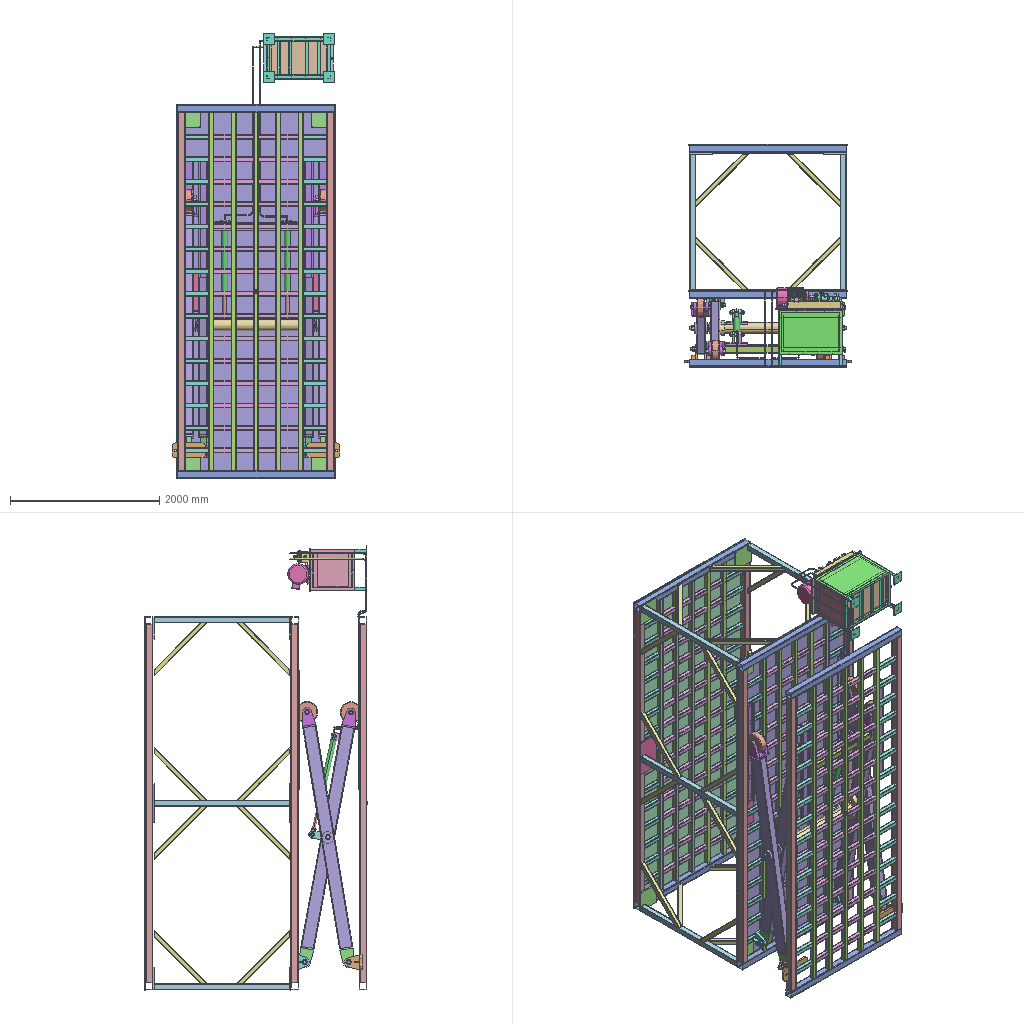Assembly | SolidWorks | 68 different items | 528 placed | box 2250 x 2986 x 5966 mm
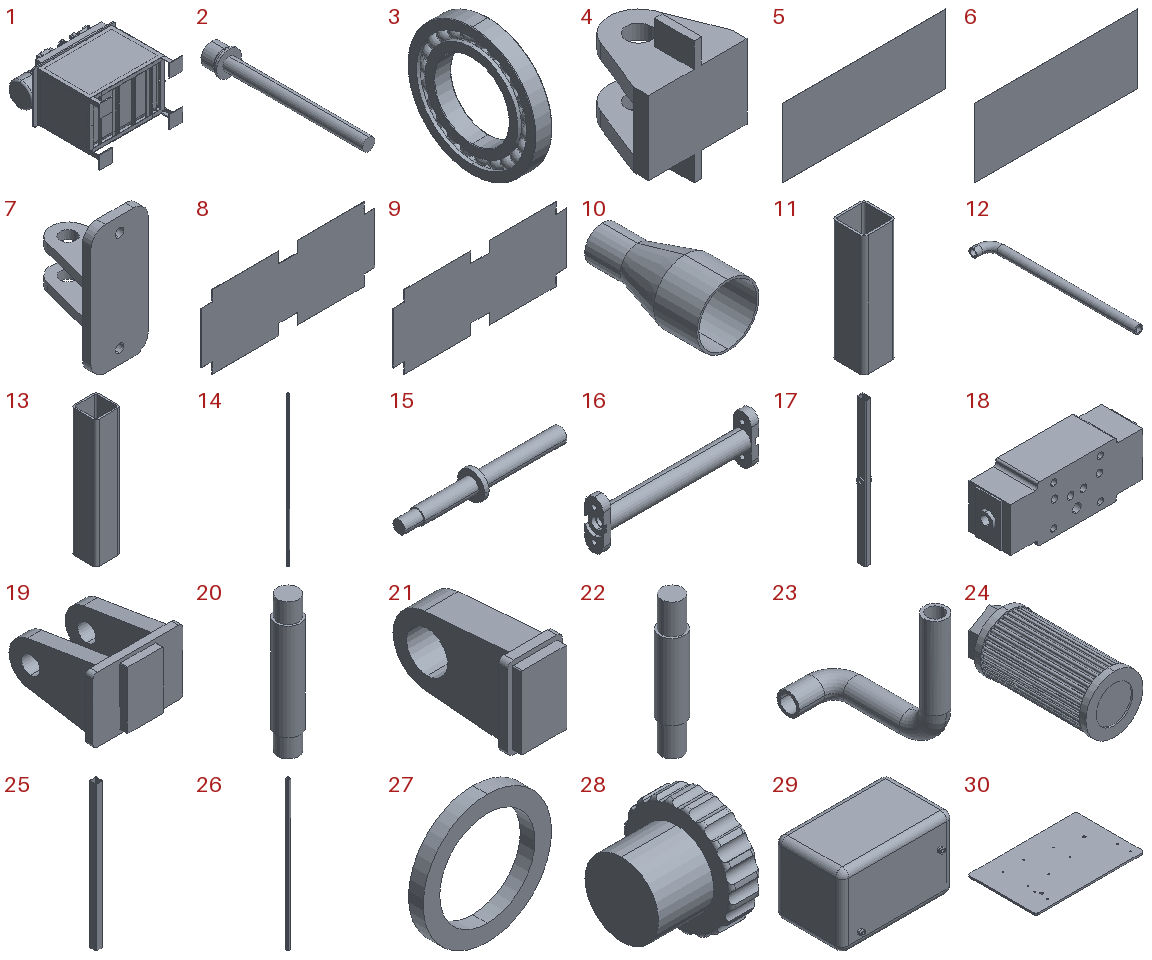Parts list (item | name | quantity | parent item | size | volume | features):
1 | (subassembly) | x1 | - | 956 x 1060 x 656 mm | 60828027 mm3 | features ReferencePattern 14, CompositeCurve 3, MirrorCompFeat 2
2 | - | x12 | in 1 | 12 x 76 x 12 mm | 2512 mm3 | features ICE 3, Revolution 1
3 | - | x18 | - | 9 x 68 x 68 mm | 16956 mm3 | features Revolution 3, CirPattern 1, Fillet 1
4 | - | x2 | - | 200 x 180 x 250 mm | 2133825 mm3 | features ICE 2, Extrusion 1, MirrorPattern 1
5 | - | x1 | - | 5020 x 8 x 2120 mm | 85139200 mm3 | features Extrusion 1
6 | - | x1 | - | 5020 x 3 x 2120 mm | 31927200 mm3 | features Extrusion 1
7 | - | x2 | - | 200 x 240 x 450 mm | 4353229 mm3 | features ICE 3, Extrusion 1, Fillet 1, MirrorPattern 1
8 | - | x1 | - | 5020 x 8 x 2120 mm | 79292800 mm3 | features Extrusion 1
9 | - | x1 | - | 5020 x 3 x 2120 mm | 29734800 mm3 | features Extrusion 1
10 | - | x1 | in 1 | 45 x 91 x 45 mm | 14846 mm3 | features Revolution 1
11 | - | x180 | - | 64 x 64 x 236 mm | 216836 mm3 | features Extrusion 1
12 | - | x1 | in 1 | 56 x 411 x 22 mm | 77381 mm3 | features Sweep 1
13 | - | x91 | - | 64 x 64 x 326 mm | 299528 mm3 | features Extrusion 1
14 | - | x18 | - | 64 x 64 x 4800 mm | 4410223 mm3 | features Extrusion 1
15 | - | x2 | - | 535 x 90 x 90 mm | 1081760 mm3 | features ICE 2, Revolution 1
16 | - | x1 | - | 1290 x 150 x 400 mm | 20836949 mm3 | features ICE 4, MirrorPattern 1, Revolution 1
17 | - | x4 | - | 170 x 180 x 3000 mm | 17246858 mm3 | features ICE 2, Extrusion 1, MirrorPattern 1
18 | - | x2 | in 1 | 164 x 48.5 x 64 mm | 411589 mm3 | features ICE 4, Extrusion 1, MirrorPattern 1
19 | - | x4 | - | 250 x 280 x 180 mm | 3684479 mm3 | features ICE 2, Extrusion 1, MirrorPattern 1
20 | - | x4 | - | 50 x 50 x 276 mm | 495680 mm3 | features Extrusion 1, ICE 1, MirrorPattern 1
21 | - | x4 | - | 120 x 295 x 180 mm | 3133759 mm3 | features ICE 2, Extrusion 1
22 | - | x4 | - | 50 x 50 x 270 mm | 460777 mm3 | features Extrusion 1, ICE 1, MirrorPattern 1
23 | - | x1 | in 1 | 56 x 122 x 116.5 mm | 41399 mm3 | features Sweep 2
24 | - | x1 | in 1 | 70 x 153 x 70 mm | 294269 mm3 | features ICE 2, Revolution 1, SweepThread 1
25 | - | x10 | - | 100 x 100 x 2100 mm | 3854801 mm3 | features Extrusion 1
26 | - | x6 | - | 100 x 100 x 4800 mm | 8810973 mm3 | features Extrusion 1
27 | - | x16 | - | 70 x 8 x 70 mm | 13798 mm3 | features Extrusion 1
28 | - | x1 | in 1 | 23 x 29.813 x 29.813 mm | 9978 mm3 | features ICE 1, Revolution 1
29 | - | x1 | in 1 | 883.103 x 546.258 x 540 mm | 6439687 mm3 | features ICE 6, Fillet 2, Extrusion 1, Shell 1
30 | - | x1 | in 1 | 930 x 586 x 15 mm | 8146365 mm3 | features Extrusion 1
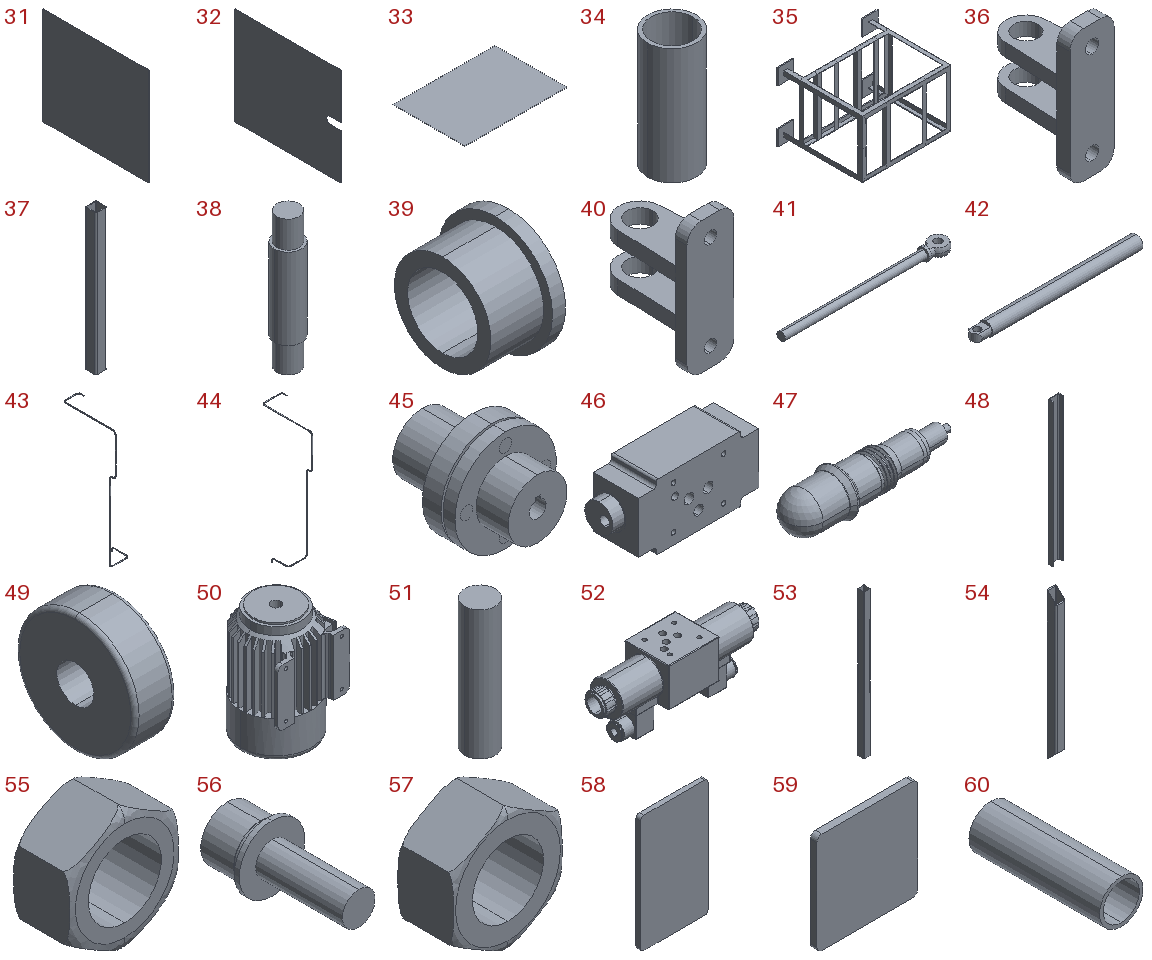31 | - | x1 | in 1 | 2 x 600 x 554 mm | 664800 mm3 | features FlatPattern 1, SMBaseFlange 1, SheetMetal 1
32 | - | x1 | in 1 | 2 x 600 x 554 mm | 658743 mm3 | features FlatPattern 1, SMBaseFlange 1, SheetMetal 1
33 | - | x2 | in 1 | 850 x 600 x 2 mm | 1020000 mm3 | features FlatPattern 1, SMBaseFlange 1, SheetMetal 1
34 | - | x1 | in 1 | 42 x 42 x 100 mm | 36757 mm3 | features Extrusion 1
35 | - | x1 | in 1 | 956 x 760 x 656 mm | 4250564 mm3 | features ICE 4, MirrorSolid 1, Sweep 1
36 | - | x2 | - | 100 x 195 x 300 mm | 1566993 mm3 | features ICE 3, Extrusion 1, Fillet 1, MirrorPattern 1
37 | - | x1 | - | 100 x 100 x 1290 mm | 2367949 mm3 | features Extrusion 1
38 | - | x4 | - | 40 x 40 x 200 mm | 219220 mm3 | features Extrusion 1, ICE 1, MirrorPattern 1
39 | - | x8 | - | 37.5 x 65 x 65 mm | 49038 mm3 | features Revolution 1
40 | - | x2 | - | 100 x 195 x 280 mm | 1415210 mm3 | features ICE 3, Extrusion 1, Fillet 1, MirrorPattern 1
41 | - | x2 | - | 900 x 100 x 65 mm | 1587827 mm3 | features ICE 2, Revolution 1
42 | - | x2 | - | 968 x 80 x 80 mm | 3418828 mm3 | features ICE 2, Revolution 1
43 | - | x1 | - | 377.2 x 1030 x 2425 mm | 462848 mm3 | features Sweep 5
44 | - | x1 | - | 790.937 x 1030 x 2325 mm | 464272 mm3 | features Sweep 5
45 | - | x1 | in 1 | 120 x 136.5 x 120 mm | 665087 mm3 | features ICE 6, Revolution 1
46 | - | x1 | in 1 | 153.5 x 48.5 x 70 mm | 400500 mm3 | features ICE 4, 3DProfileFeature 1, Extrusion 1, HoleWzd 1, MirrorPattern 1
47 | - | x1 | in 1 | 144.393 x 39.501 x 39.501 mm | 86729 mm3 | features Fillet 1, Revolution 1, SweepThread 1
48 | - | x4 | - | 120 x 53 x 1600 mm | 2068917 mm3 | features Extrusion 1
49 | - | x4 | - | 100 x 289 x 289 mm | 5885186 mm3 | features Fillet 1, Revolution 1
50 | - | x1 | in 1 | 350 x 284.5 x 435 mm | 22165719 mm3 | features ICE 6, Fillet 2, Revolution 1
51 | - | x1 | in 1 | 38 x 38 x 160 mm | 178690 mm3 | features Extrusion 1, ICE 1
52 | - | x1 | in 1 | 283 x 80 x 110 mm | 1025505 mm3 | features ICE 10, Extrusion 1, Fillet 1, MirrorPattern 1, Revolution 1
53 | - | x6 | - | 81 x 81 x 1811 mm | 2181406 mm3 | features Extrusion 1
54 | - | x24 | - | 64 x 64 x 1007 mm | 866205 mm3 | features Extrusion 1, ICE 1
55 | - | x8 | - | 49 x 26 x 56.58 mm | 31477 mm3 | features Extrusion 1, RevCut 1
56 | - | x6 | in 1 | 20 x 40 x 20 mm | 4696 mm3 | features ICE 3, Revolution 1
57 | - | x18 | - | 64 x 33 x 73.901 mm | 71017 mm3 | features Extrusion 1, RevCut 1
58 | - | x4 | - | 300 x 20 x 520 mm | 3116137 mm3 | features Extrusion 1
59 | - | x8 | - | 300 x 20 x 300 mm | 1796137 mm3 | features Extrusion 1
60 | - | x4 | - | 60 x 180 x 60 mm | 155509 mm3 | features Extrusion 1
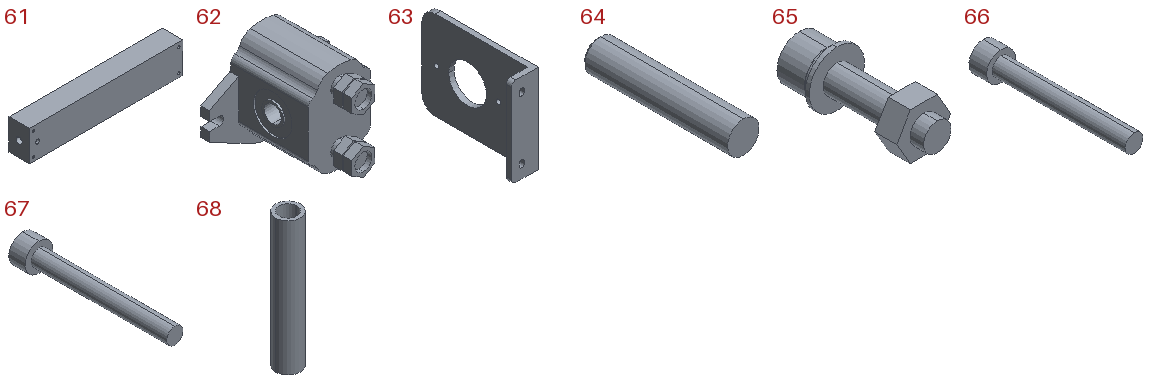61 | - | x1 | in 1 | 750 x 100 x 150 mm | 11136874 mm3 | features 3DProfileFeature 2, HoleWzd 2, Extrusion 1, ICE 1, RevCut 1
62 | - | x1 | in 1 | 155 x 138.5 x 127 mm | 875484 mm3 | features ICE 9, Extrusion 1, MirrorPattern 1
63 | - | x1 | in 1 | 60 x 250 x 200 mm | 636149 mm3 | features Fillet 2, ICE 2, Extrusion 1
64 | - | x1 | in 1 | 20 x 92.5 x 20 mm | 28405 mm3 | features Chamfer 1, Extrusion 1, ICE 1
65 | - | x2 | in 1 | 20 x 50 x 20 mm | 6831 mm3 | features ICE 4, Revolution 1
66 | - | x4 | in 1 | 16.2 x 85 x 16.2 mm | 7619 mm3 | features ICE 1, Revolution 1
67 | - | x4 | in 1 | 10.2 x 56 x 10.2 mm | 1796 mm3 | features ICE 1, Revolution 1
68 | - | x1 | in 1 | 22 x 22 x 120 mm | 21488 mm3 | features Extrusion 1
Mates (type | each side: item.copy, entity, surface, feature):
In the top assembly
Coincident | 26.1 face plane Boss-Extrude 1 | 25.1 face plane Boss-Extrude 1 | 3 times
Coincident | 26.1 face plane Boss-Extrude 1 | 25.2 face plane Boss-Extrude 1 | 3 times
Coincident | 25.1 face plane Boss-Extrude 1 | 14.1 face plane Boss-Extrude 1 | 2 times
Width | 14.1 face plane Boss-Extrude 1 | 14.1 face plane Boss-Extrude 1 | 25.1 face plane Boss-Extrude 1 | 25.1 face plane Boss-Extrude 1
Coincident | 14.1 face plane Boss-Extrude 1 | 11.1 face plane Boss-Extrude 1 | 2 times
Coincident | 14.1 plane | assembly plane | 3 times
DistanceDim | 11.1 face plane Boss-Extrude 1 | 25.1 face plane Boss-Extrude 1
Coincident | 11.1 face plane Boss-Extrude 1 | 13.1 face plane Boss-Extrude 1 | 2 times
Coincident | 26.1 face plane Boss-Extrude 1 | 13.1 face plane Boss-Extrude 1
Coincident | 14.1 face plane Boss-Extrude 1 | 7.1 face plane Boss-Extrude 1
Width | 7.1 face plane Boss-Extrude 1 | 7.1 face plane Boss-Extrude 1 | 13.1 face plane Boss-Extrude 1 | 13.1 face plane Boss-Extrude 1
Width | 21.1 face plane Boss-Extrude 2 | 21.1 face plane Boss-Extrude 2 | 17.1 face plane Boss-Extrude 1 | 17.1 face plane Boss-Extrude 1 | 2 times
Coincident | 17.1 face plane Boss-Extrude 1 | 21.1 face plane Boss-Extrude 1
Width | 21.1 face plane Boss-Extrude 3 | 21.1 face plane Boss-Extrude 3 | 7.1 face plane Boss-Extrude 1 | 7.1 face plane Boss-Extrude 1
Concentric | 7.1 face cylinder Mirror 1 | 21.1 face cylinder Boss-Extrude 3
Width | 7.1 face plane Boss-Extrude 1 | 7.1 face plane Boss-Extrude 1 | assembly face | assembly face
Concentric | 21.1 face cylinder Boss-Extrude 3 | 3.1 face cylinder Revolve2
Coincident | 21.1 face plane Boss-Extrude 3 | 3.1 face plane Revolve3
Concentric | 7.1 face cylinder Mirror 1 | 22.1 face cylinder Boss-Extrude 1
Width | 22.1 face plane Boss-Extrude 1 | 22.1 face plane Boss-Extrude 1 | 7.1 face plane Boss-Extrude 1 | 7.1 face plane Boss-Extrude 1
Concentric | 22.1 face cylinder Boss-Extrude 2 | 57.1 face cylinder Boss-Extrude 1
Coincident | 7.1 face plane Boss-Extrude 1 | 57.1 face plane Boss-Extrude 1
Width | 19.1 face plane Boss-Extrude 2 | 19.1 face plane Boss-Extrude 2 | 17.1 face plane Boss-Extrude 1 | 17.1 face plane Boss-Extrude 1
Width | 17.1 face plane Boss-Extrude 1 | 17.1 face plane Boss-Extrude 1 | 19.1 face plane Boss-Extrude 2 | 19.1 face plane Boss-Extrude 2
Coincident | 17.1 face plane Boss-Extrude 1 | 19.1 face plane Boss-Extrude 1
Coincident | 21.1 face plane Boss-Extrude 3 | 27.1 face plane Boss-Extrude 1
Concentric | 22.1 face cylinder Boss-Extrude 2 | 27.1 face cylinder Boss-Extrude 1
Concentric | 19.1 face cylinder Mirror 1 | 49.1 face cylinder Revolve 1
Width | 49.1 face plane Revolve 1 | 49.1 face plane Revolve 1 | 19.1 face plane Boss-Extrude 3 | 19.1 face plane Mirror 1
Coincident | 49.1 face plane Revolve 1 | 3.2 face plane Revolve3
Concentric | 49.1 face cylinder Revolve 1 | 3.2 face cylinder Revolve3
Coincident | 49.1 face plane Revolve 1 | 27.2 face plane Boss-Extrude 1
Concentric | 3.2 face cylinder Revolve2 | 27.2 face cylinder Boss-Extrude 1
Concentric | 17.1 face cylinder Cut-Extrude 1 | 60.1 face cylinder Boss-Extrude 1
Concentric | 60.1 face cylinder Boss-Extrude 1 | 15.1 face cylinder Revolve 1
Width | 60.1 face plane Boss-Extrude 1 | 60.1 face plane Boss-Extrude 1 | 17.1 face plane Mirror 1 | 17.1 face plane Boss-Extrude 2
Coincident | 60.1 face plane Boss-Extrude 1 | 15.1 face plane Revolve 1
Concentric | 15.1 face cylinder Boss-Extrude 2 | 57.2 face cylinder Boss-Extrude 1
Coincident | 15.1 face plane Revolve 1 | 57.2 face plane Boss-Extrude 1
Concentric | 17.2 face cylinder Cut-Extrude 1 | 60.2 face cylinder Boss-Extrude 1
Width | 17.2 face plane Boss-Extrude 2 | 17.2 face plane Mirror 1 | 60.2 face plane Boss-Extrude 1 | 60.2 face plane Boss-Extrude 1
Concentric | 15.1 face cylinder Revolve 1 | 60.2 face cylinder Boss-Extrude 1
Coincident | 15.1 face plane Revolve 1 | 60.2 face plane Boss-Extrude 1
Width | 21.2 face plane Boss-Extrude 2 | 21.2 face plane Boss-Extrude 2 | 17.2 face plane Boss-Extrude 1 | 17.2 face plane Boss-Extrude 1 | 2 times
Coincident | 17.2 face plane Boss-Extrude 1 | 21.2 face plane Boss-Extrude 1
Width | 20.1 face plane Boss-Extrude 1 | 20.1 face plane Boss-Extrude 1 | 19.1 face plane Mirror 1 | 19.1 face plane Boss-Extrude 3
Concentric | 19.1 face cylinder Boss-Extrude 3 | 20.1 face cylinder Boss-Extrude 1
Concentric | 20.1 face cylinder Boss-Extrude 2 | 57.3 face cylinder Boss-Extrude 1
Coincident | 19.1 face plane Mirror 1 | 57.3 face plane Boss-Extrude 1
Concentric | 21.2 face cylinder Boss-Extrude 3 | 22.2 face cylinder Boss-Extrude 1
Width | 21.2 face plane Boss-Extrude 3 | 21.2 face plane Boss-Extrude 3 | 22.2 face plane Boss-Extrude 1 | 22.2 face plane Boss-Extrude 1
Concentric | 21.2 face cylinder Boss-Extrude 3 | 3.3 face cylinder Revolve3
Coincident | 21.2 face plane Boss-Extrude 3 | 3.3 face plane Revolve3
Coincident | 21.2 face plane Boss-Extrude 3 | 27.3 face plane Boss-Extrude 1
Concentric | 22.2 face cylinder Boss-Extrude 1 | 27.3 face cylinder Boss-Extrude 1
Width | 4.1 face plane Boss-Extrude 2 | 4.1 face plane Mirror 1 | 21.2 face plane Boss-Extrude 3 | 21.2 face plane Boss-Extrude 3
Concentric | 22.2 face cylinder Boss-Extrude 2 | 4.1 face cylinder Mirror 1
Concentric | 22.2 face cylinder Boss-Extrude 2 | 57.4 face cylinder Boss-Extrude 1
Coincident | 4.1 face plane Boss-Extrude 1 | 57.4 face plane Boss-Extrude 1
Width | 19.2 face plane Boss-Extrude 2 | 19.2 face plane Boss-Extrude 2 | 17.2 face plane Boss-Extrude 1 | 17.2 face plane Boss-Extrude 1 | 2 times
Coincident | 17.2 face plane Boss-Extrude 1 | 19.2 face plane Boss-Extrude 1
Width | 49.2 face plane Revolve 1 | 49.2 face plane Revolve 1 | 19.2 face plane Boss-Extrude 3 | 19.2 face plane Mirror 1
Concentric | 19.2 face cylinder Mirror 1 | 49.2 face cylinder Revolve 1
Concentric | 49.2 face cylinder Revolve 1 | 20.2 face cylinder Boss-Extrude 1
Width | 20.2 face plane Boss-Extrude 2 | 20.2 face plane Mirror 1 | 19.2 face plane Boss-Extrude 3 | 19.2 face plane Mirror 1
Coincident | 49.2 face plane Revolve 1 | 3.4 face plane Revolve3
Concentric | 49.2 face cylinder Revolve 1 | 3.4 face cylinder Revolve3
Coincident | 49.2 face plane Revolve 1 | 27.4 face plane Boss-Extrude 1
Concentric | 20.2 face cylinder Boss-Extrude 2 | 27.4 face cylinder Boss-Extrude 1
Coincident | 19.2 face plane Mirror 1 | 57.5 face plane Boss-Extrude 1
Concentric | 20.2 face cylinder Boss-Extrude 2 | 57.5 face cylinder Boss-Extrude 1
Width | 16.1 face plane Revolve 1 | 16.1 face plane Revolve 1 | 14.1 face plane Boss-Extrude 1 | 14.1 face plane Boss-Extrude 1
Concentric | 15.1 face cylinder Revolve 1 | 16.1 face cylinder Revolve 1
Width | 48.1 face plane Boss-Extrude 1 | 48.1 face plane Boss-Extrude 1 | 49.2 face plane Revolve 1 | 49.2 face plane Revolve 1
Coincident | 14.1 face plane Boss-Extrude 1 | 48.1 face plane Boss-Extrude 1
Tangent | 49.2 face cylinder Revolve 1 | 48.1 face plane Boss-Extrude 1
Concentric | 42.1 face cylinder Revolve 1 | 41.1 face cylinder Revolve 1
Coincident | 17.2 face plane Boss-Extrude 1 | 37.1 face plane Boss-Extrude 1 | 2 times
DistanceDim | 37.1 face plane Boss-Extrude 1 | 19.2 face plane Boss-Extrude 1
Width | 36.1 face plane Mirror 1 | 36.1 face plane Boss-Extrude 2 | 42.1 face plane Cut-Extrude 2 | 42.1 face plane Cut-Extrude 2
Coincident | 37.1 face plane Boss-Extrude 1 | 36.1 face plane Boss-Extrude 1
Width | 36.1 face plane Boss-Extrude 1 | 36.1 face plane Boss-Extrude 1 | 37.1 face plane Boss-Extrude 1 | 37.1 face plane Boss-Extrude 1
Concentric | 42.1 face cylinder Cut-Extrude 1 | 36.1 face cylinder Mirror 1
DistanceDim | 36.1 plane | assembly plane
Width | 41.1 face plane Cut-Extrude 1 | 41.1 face plane Cut-Extrude 1 | 40.1 face plane Boss-Extrude 2 | 40.1 face plane Mirror 1
Concentric | 41.1 face cylinder Cut-Extrude 2 | 40.1 face cylinder Boss-Extrude 2
Coincident | 16.1 face plane Cut-Extrude 1 | 40.1 face plane Boss-Extrude 1
Coincident | 16.1 plane | 40.1 plane
Coincident | 26.2 face plane Boss-Extrude 1 | 25.3 face plane Boss-Extrude 1 | 3 times
Coincident | 26.2 face plane Boss-Extrude 1 | 25.4 face plane Boss-Extrude 1 | 3 times
Width | 14.2 face plane Boss-Extrude 1 | 14.2 face plane Boss-Extrude 1 | 25.3 face plane Boss-Extrude 1 | 25.3 face plane Boss-Extrude 1
Coincident | 25.3 face plane Boss-Extrude 1 | 14.2 face plane Boss-Extrude 1 | 2 times
Coincident | 25.1 face plane Boss-Extrude 1 | 25.3 face plane Boss-Extrude 1
Coincident | 26.1 face plane Boss-Extrude 1 | 26.2 face plane Boss-Extrude 1
Coincident | 14.2 face plane Boss-Extrude 1 | 11.2 face plane Boss-Extrude 1 | 2 times
Coincident | 11.1 face plane Boss-Extrude 1 | 11.2 face plane Boss-Extrude 1
Coincident | 26.2 face plane Boss-Extrude 1 | 13.2 face plane Boss-Extrude 1 | 2 times
Coincident | 11.2 face plane Boss-Extrude 1 | 13.2 face plane Boss-Extrude 1
Coincident | 4.1 face plane Boss-Extrude 1 | 14.2 face plane Boss-Extrude 1
Coincident | 14.2 face plane Boss-Extrude 1 | 48.2 face plane Boss-Extrude 1
Coincident | 48.1 face plane Boss-Extrude 1 | 48.2 face plane Boss-Extrude 1
Width | 48.2 face plane Boss-Extrude 1 | 48.2 face plane Boss-Extrude 1 | 49.1 face plane Revolve 1 | 49.1 face plane Revolve 1
Coincident | 26.2 face plane Boss-Extrude 1 | 59.1 face plane Boss-Extrude 1 | 2 times
Coincident | 25.4 face plane Boss-Extrude 1 | 59.1 face plane Boss-Extrude 1
Coincident | 26.2 face plane Boss-Extrude 1 | 59.2 face plane Boss-Extrude 1 | 2 times
Coincident | 25.3 face plane Boss-Extrude 1 | 59.2 face plane Boss-Extrude 1
Coincident | 26.2 face plane Boss-Extrude 1 | 58.1 face plane Boss-Extrude 1 | 2 times
Width | 58.1 face plane Boss-Extrude 1 | 58.1 face plane Boss-Extrude 1 | 25.3 face plane Boss-Extrude 1 | 25.4 face plane Boss-Extrude 1
Width | 8.1 face plane Boss-Extrude 1 | 8.1 face plane Boss-Extrude 1 | 25.3 face plane Boss-Extrude 1 | 25.4 face plane Boss-Extrude 1
Width | 8.1 face plane Boss-Extrude 1 | 8.1 face plane Boss-Extrude 1 | 25.4 face plane Boss-Extrude 1 | 25.4 face plane Boss-Extrude 1
Coincident | 26.2 face plane Boss-Extrude 1 | 8.1 face plane Boss-Extrude 1
Coincident | 9.1 face plane Boss-Extrude 1 | 8.1 face plane Boss-Extrude 1 | 3 times
Coincident | 59.1 face plane Boss-Extrude 1 | 53.1 face plane Boss-Extrude 1 | 3 times
Coincident | 58.1 face plane Boss-Extrude 1 | 53.2 face plane Boss-Extrude 1 | 2 times
Width | 53.2 face plane Boss-Extrude 1 | 53.2 face plane Boss-Extrude 1 | 58.1 face plane Boss-Extrude 1 | 58.1 face plane Boss-Extrude 1
Coincident | 59.2 face plane Boss-Extrude 1 | 53.3 face plane Boss-Extrude 1 | 3 times
Width | 54.1 face plane Boss-Extrude 1 | 54.1 face plane Boss-Extrude 1 | 53.1 face plane Boss-Extrude 1 | 53.1 face plane Boss-Extrude 1
Coincident | 53.1 face plane Boss-Extrude 1 | 54.1 face plane Cut-Extrude 1
Coincident | 59.1 face plane Boss-Extrude 1 | 54.1 face plane Cut-Extrude 1
Width | 54.2 face plane Boss-Extrude 1 | 54.2 face plane Boss-Extrude 1 | 53.1 face plane Boss-Extrude 1 | 53.1 face plane Boss-Extrude 1
Coincident | 59.1 face plane Boss-Extrude 1 | 54.2 face plane Cut-Extrude 1
Coincident | 53.1 face plane Boss-Extrude 1 | 54.2 face plane Cut-Extrude 1
Coincident | 58.1 face plane Boss-Extrude 1 | 54.3 face plane Cut-Extrude 1
Coincident | 53.2 face plane Boss-Extrude 1 | 54.3 face plane Cut-Extrude 1
Width | 54.3 face plane Boss-Extrude 1 | 54.3 face plane Boss-Extrude 1 | 53.2 face plane Boss-Extrude 1 | 53.2 face plane Boss-Extrude 1
Coincident | 58.1 face plane Boss-Extrude 1 | 54.4 face plane Cut-Extrude 1
Coincident | 53.2 face plane Boss-Extrude 1 | 54.4 face plane Cut-Extrude 1
Width | 54.4 face plane Boss-Extrude 1 | 54.4 face plane Boss-Extrude 1 | 53.2 face plane Boss-Extrude 1 | 53.2 face plane Boss-Extrude 1
Coincident | 59.2 face plane Boss-Extrude 1 | 54.5 face plane Cut-Extrude 1
Coincident | 53.3 face plane Boss-Extrude 1 | 54.5 face plane Cut-Extrude 1
Width | 53.3 face plane Boss-Extrude 1 | 53.3 face plane Boss-Extrude 1 | 54.5 face plane Boss-Extrude 1 | 54.5 face plane Boss-Extrude 1
Coincident | 59.2 face plane Boss-Extrude 1 | 54.6 face plane Cut-Extrude 1
Coincident | 53.3 face plane Boss-Extrude 1 | 54.6 face plane Cut-Extrude 1
Width | 53.3 face plane Boss-Extrude 1 | 53.3 face plane Boss-Extrude 1 | 54.6 face plane Boss-Extrude 1 | 54.6 face plane Boss-Extrude 1
Width | 14.3 face plane Boss-Extrude 1 | 14.3 face plane Boss-Extrude 1 | 25.4 face plane Boss-Extrude 1 | 25.4 face plane Boss-Extrude 1
Coincident | 25.5 face plane Boss-Extrude 1 | 14.3 face plane Boss-Extrude 1 | 2 times
Coincident | 14.4 face plane Boss-Extrude 1 | 11.3 face plane Boss-Extrude 1
Coincident | 14.3 face plane Boss-Extrude 1 | 11.3 face plane Boss-Extrude 1
Coincident | 11.2 face plane Boss-Extrude 1 | 11.3 face plane Boss-Extrude 1
Coincident | 13.3 face plane Boss-Extrude 1 | 11.3 face plane Boss-Extrude 1 | 2 times
Coincident | 26.3 face plane Boss-Extrude 1 | 13.3 face plane Boss-Extrude 1
Width | 6.1 face plane Boss-Extrude 1 | 6.1 face plane Boss-Extrude 1 | 25.6 face plane Boss-Extrude 1 | 25.5 face plane Boss-Extrude 1
Width | 25.5 face plane Boss-Extrude 1 | 25.5 face plane Boss-Extrude 1 | 6.1 face plane Boss-Extrude 1 | 6.1 face plane Boss-Extrude 1
Coincident | 25.5 face plane Boss-Extrude 1 | 5.1 face plane Boss-Extrude 1
Width | 5.1 face plane Boss-Extrude 1 | 5.1 face plane Boss-Extrude 1 | 25.6 face plane Boss-Extrude 1 | 25.5 face plane Boss-Extrude 1
Width | 5.1 face plane Boss-Extrude 1 | 5.1 face plane Boss-Extrude 1 | 25.5 face plane Boss-Extrude 1 | 25.5 face plane Boss-Extrude 1
Coincident | 6.1 face plane Boss-Extrude 1 | 5.1 face plane Boss-Extrude 1
Concentric | 36.1 face cylinder Boss-Extrude 2 | 39.1 face cylinder Revolve 1
Coincident | 36.1 face plane Boss-Extrude 2 | 39.1 face plane Revolve 1
Concentric | 42.1 face cylinder Cut-Extrude 1 | 38.1 face cylinder Boss-Extrude 1
Width | 38.1 face plane Mirror 1 | 38.1 face plane Boss-Extrude 2 | 36.1 face plane Boss-Extrude 1 | 36.1 face plane Boss-Extrude 1
Concentric | 40.1 face cylinder Boss-Extrude 2 | 39.2 face cylinder Revolve 1
Coincident | 40.1 face plane Boss-Extrude 2 | 39.2 face plane Revolve 1
Concentric | 40.1 face cylinder Mirror 1 | 38.2 face cylinder Boss-Extrude 1
Width | 38.2 face plane Mirror 1 | 38.2 face plane Boss-Extrude 2 | 40.1 face plane Boss-Extrude 1 | 40.1 face plane Boss-Extrude 1
Concentric | 38.1 face cylinder Boss-Extrude 2 | 55.1 face cylinder Boss-Extrude 1
Coincident | 39.1 face plane Revolve 1 | 55.1 face plane Boss-Extrude 1
Concentric | 38.2 face cylinder Boss-Extrude 2 | 55.2 face cylinder Boss-Extrude 1
Coincident | 40.1 face plane Boss-Extrude 1 | 55.2 face plane Boss-Extrude 1
Parallel | 17.2 face plane Boss-Extrude 1 | 16.1 face plane Boss-Extrude 1
DistanceDim | 48.1 face plane Boss-Extrude 1 | 25.2 face plane Boss-Extrude 1
Coincident | 25.2 face plane Boss-Extrude 1 | 35.1 face plane Boss-Extrude 3
Coincident | 26.4 face plane Boss-Extrude 1 | 35.1 face plane Boss-Extrude 3
DistanceDim | 25.2 face plane Boss-Extrude 1 | 35.1 face plane Boss-Extrude 3
Coincident | 18.1 face plane Boss-Extrude 1 | 43.1 face plane Sweep 1
Concentric | 18.1 face cylinder Cut-Extrude 1 | 43.1 face cylinder Sweep 1
Parallel | 33.1 face plane Base-Flange 1 | 43.1 plane
Coincident | 18.2 face plane Boss-Extrude 1 | 44.1 face plane Sweep 1
Concentric | 18.2 face cylinder Cut-Extrude 1 | 44.1 face cylinder Sweep 1
Parallel | 33.1 face plane Base-Flange 1 | 44.1 plane
In subassembly 1
Concentric | 45.1 face cylinder Revolve 1 | 51.1 face cylinder Boss-Extrude 1
Coincident | 45.1 face plane Cut-Extrude 3 | 51.1 face plane Cut-Extrude 1
Coincident | 62.1 face plane Cut-Extrude 1 | 64.1 face plane Boss-Extrude 1
Concentric | 62.1 face cylinder Cut-Extrude 1 | 64.1 face cylinder Boss-Extrude 1
Concentric | 45.1 face cylinder Boss-Extrude 2 | 64.1 face cylinder Boss-Extrude 1
Coincident | 45.1 face plane Cut-Extrude 2 | 64.1 face plane Cut-Extrude 1
DistanceDim | 45.1 face plane Boss-Extrude 3 | 62.1 face plane Boss-Extrude 3
Concentric | 51.1 face cylinder Boss-Extrude 1 | 50.1 face cylinder Revolve 1
Coincident | 51.1 face plane Boss-Extrude 1 | 50.1 face plane Revolve 1
DistanceDim | 50.1 face plane Revolve 1 | 45.1 face plane Revolve 1
Coincident | 30.1 face plane Boss-Extrude 1 | 1.1 plane
Coincident | 30.1 plane | 1.1 plane | 2 times
Coincident | 50.1 face plane Boss-Extrude 1 | 30.1 face plane Boss-Extrude 1
Concentric | 50.1 face cylinder Cut-Extrude 2 | 30.1 face cylinder Boss-Extrude 1 | 2 times
Coincident | 30.1 face plane Boss-Extrude 1 | 61.1 face plane Boss-Extrude 1
Concentric | 30.1 face cylinder Boss-Extrude 1 | 61.1 face cylinder Boss-Extrude 1 | 2 times
Coincident | 52.1 face plane Boss-Extrude 1 | 61.1 face plane Boss-Extrude 1
Concentric | 52.1 face cylinder Cut-Extrude 4 | 61.1 face cylinder M6 threaded hole 1 | 2 times
Coincident | 18.3 face plane Boss-Extrude 1 | 61.1 face plane Boss-Extrude 1
Concentric | 47.1 face cylinder Revolve 1 | 61.1 face cylinder Cut-Revolve 1
Coincident | 47.1 edge | 61.1 face plane Boss-Extrude 1
Concentric | 62.1 face cylinder Boss-Extrude 3 | 63.1 face cylinder Cut-Extrude 2
Tangent | 30.1 face cylinder Boss-Extrude 1 | 63.1 face plane Cut-Extrude 1
Coincident | 30.1 face plane Boss-Extrude 1 | 63.1 face plane Boss-Extrude 1
Concentric | 24.1 face cylinder Revolve 1 | 30.1 face cylinder Boss-Extrude 1
Coincident | 24.1 face plane Revolve 1 | 34.1 face plane Boss-Extrude 1
Concentric | 24.1 face cylinder Revolve 1 | 34.1 face cylinder Boss-Extrude 1
Coincident | 34.1 face plane Boss-Extrude 1 | 10.1 edge
Concentric | 34.1 face cylinder Boss-Extrude 1 | 10.1 face cylinder Revolve 1
Concentric | 10.1 face cylinder Revolve 1 | 12.1 face cylinder Sweep 1
Concentric | 62.1 face cylinder Boss-Extrude 4 | 12.1 face cylinder Sweep 1
Coincident | 10.1 edge | 12.1 face plane Sweep 1
Concentric | 62.1 face cylinder Boss-Extrude 4 | 23.1 face cylinder Sweep 1
Coincident | 61.1 face plane Boss-Extrude 1 | 23.1 face plane Sweep 2
Concentric | 30.1 face cylinder Boss-Extrude 1 | 68.1 face cylinder Boss-Extrude 1
DistanceDim | 61.1 face plane Boss-Extrude 1 | 68.1 face plane Boss-Extrude 1
Coincident | 30.1 face plane Boss-Extrude 1 | 35.2 face plane Mirror 4
Width | 35.2 face plane Sweep 1 | 35.2 face plane Sweep 1 | 30.1 face plane Boss-Extrude 1 | 30.1 face plane Boss-Extrude 1 | 2 times
Coincident | 62.1 face plane Cut-Extrude 4 | 23.1 face plane Sweep 1
Concentric | 12.1 face cylinder Sweep 1 | 29.1 face cylinder Boss-Extrude 2
Concentric | 68.1 face cylinder Boss-Extrude 1 | 29.1 face cylinder Boss-Extrude 2
Coincident | 35.2 face plane Boss-Extrude 4 | 29.1 face plane Boss-Extrude 1
Concentric | 29.1 face cylinder Boss-Extrude 6 | 28.1 face cylinder Revolve 1
Coincident | 29.1 face plane Boss-Extrude 6 | 28.1 face plane Revolve 1
Coincident | 35.2 face plane Sweep 1 | 33.2 face plane Base-Flange 1
Coincident | 30.1 face plane Boss-Extrude 1 | 33.2 face plane Base-Flange 1
Width | 33.2 face plane Base-Flange 1 | 33.2 face plane Base-Flange 1 | 35.2 face plane Sweep 1 | 35.2 face plane Sweep 1
Coincident | 35.2 face plane Sweep 1 | 33.3 face plane Base-Flange 1 | 2 times
Coincident | 30.1 face plane Boss-Extrude 1 | 33.3 face plane Base-Flange 1
Coincident | 35.2 face plane Sweep 1 | 31.1 face plane Base-Flange 1
Coincident | 30.1 face plane Boss-Extrude 1 | 31.1 face plane Base-Flange 1
Width | 31.1 face plane Base-Flange 1 | 31.1 face plane Base-Flange 1 | 33.3 face plane Base-Flange 1 | 33.2 face plane Base-Flange 1
Coincident | 35.2 face plane Sweep 1 | 32.1 face plane Base-Flange 1
Coincident | 30.1 face plane Boss-Extrude 1 | 32.1 face plane Base-Flange 1
Width | 32.1 face plane Base-Flange 1 | 32.1 face plane Base-Flange 1 | 33.2 face plane Base-Flange 1 | 33.3 face plane Base-Flange 1
Coincident | 63.1 face plane Boss-Extrude 1 | 56.1 face plane Boss-Extrude 2
Concentric | 30.1 face cylinder Boss-Extrude 1 | 56.1 face cylinder Revolve 1
Concentric | 50.1 face cylinder Cut-Extrude 2 | 56.2 face cylinder Revolve 1
Coincident | 50.1 face plane Boss-Extrude 1 | 56.2 face plane Boss-Extrude 2
Concentric | 50.1 face cylinder Cut-Extrude 2 | 56.3 face cylinder Revolve 1
Coincident | 50.1 face plane Boss-Extrude 1 | 56.3 face plane Boss-Extrude 2
Concentric | 63.1 face cylinder Cut-Extrude 2 | 65.1 face cylinder Revolve 1
Coincident | 62.1 face plane Boss-Extrude 2 | 65.1 face plane Boss-Extrude 2
Concentric | 63.1 face cylinder Cut-Extrude 2 | 65.2 face cylinder Revolve 1
Coincident | 62.1 face plane Boss-Extrude 2 | 65.2 face plane Boss-Extrude 2
Coincident | 61.1 face plane Cut-Extrude 1 | 66.1 face plane Revolve 1
Concentric | 61.1 face cylinder Boss-Extrude 1 | 66.1 face cylinder Revolve 1
Coincident | 61.1 face plane Cut-Extrude 1 | 66.2 face plane Revolve 1
Concentric | 61.1 face cylinder Cut-Extrude 1 | 66.2 face cylinder Revolve 1
Coincident | 18.3 face plane Boss-Extrude 1 | 2.1 face plane Boss-Extrude 2
Concentric | 18.3 face cylinder Cut-Extrude 1 | 2.1 face cylinder Revolve 1
Concentric | 18.3 face cylinder Cut-Extrude 1 | 2.2 face cylinder Revolve 1
Coincident | 18.3 face plane Boss-Extrude 1 | 2.2 face plane Boss-Extrude 2
Coincident | 52.1 face plane Cut-Extrude 3 | 67.1 face plane Revolve 1
Concentric | 52.1 face cylinder Cut-Extrude 3 | 67.1 face cylinder Revolve 1
Coincident | 52.1 face plane Cut-Extrude 3 | 67.2 face plane Revolve 1
Concentric | 52.1 face cylinder Cut-Extrude 3 | 67.2 face cylinder Revolve 1
Concentric | 18.3 face cylinder Cut-Extrude 1 | 61.1 face cylinder M6 threaded hole 1 | 2 times
Coincident | 18.3 face plane Boss-Extrude 1 | 2.3 face plane Boss-Extrude 2
Concentric | 18.3 face cylinder Cut-Extrude 1 | 2.3 face cylinder Revolve 1
Coincident | 18.3 face plane Boss-Extrude 1 | 2.4 face plane Boss-Extrude 2
Concentric | 18.3 face cylinder Cut-Extrude 1 | 2.4 face cylinder Revolve 1
Coincident | 61.1 face plane Boss-Extrude 1 | 46.1 face plane Boss-Extrude 1
Concentric | 61.1 face cylinder M6 threaded hole 1 | 46.1 face cylinder M6 threaded hole 1 | 2 times
Coincident | 46.1 face plane Boss-Extrude 1 | 2.5 face plane Boss-Extrude 2
Concentric | 46.1 face cylinder M6 threaded hole 1 | 2.5 face cylinder Revolve 1
Coincident | 46.1 face plane Boss-Extrude 1 | 2.6 face plane Boss-Extrude 2
Concentric | 46.1 face cylinder M6 threaded hole 1 | 2.6 face cylinder Revolve 1